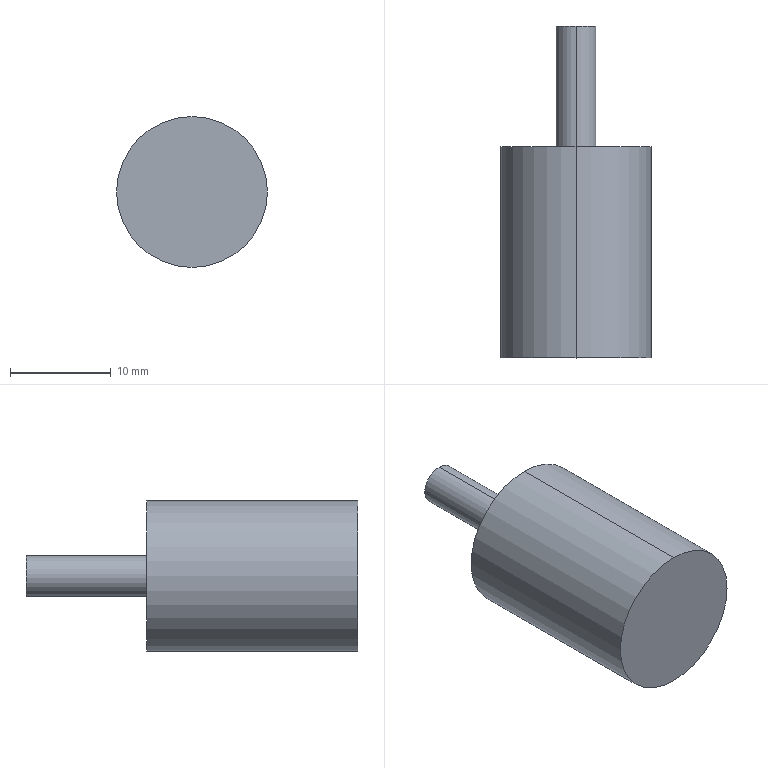Part | SolidWorks | features Revolution 1 | 1 solid | 7 faces | box 15 x 33 x 15 mm | volume 3862 mm3 | cylinder 4 | plane 3 | commonest cylinder face diameters 4 x2 15 x2
STEP:
#1=CARTESIAN_POINT('',(0.,-0.0007358,-0.0075));
#2=VERTEX_POINT('',#1);
#3=CARTESIAN_POINT('',(0.,-0.0007358,0.0075));
#4=VERTEX_POINT('',#3);
#5=CARTESIAN_POINT('',(0.,-0.0007358,0.));
#6=DIRECTION('',(0.,-1.,0.));
#7=DIRECTION('',(0.,0.,-1.));
#8=AXIS2_PLACEMENT_3D('',#5,#6,#7);
#9=CIRCLE('',#8,0.0075);
#10=EDGE_CURVE('',#2,#4,#9,.T.);
#11=ORIENTED_EDGE('',*,*,#10,.T.);
#12=CARTESIAN_POINT('',(0.,-0.02174,0.0075));
#13=VERTEX_POINT('',#12);
#14=CARTESIAN_POINT('',(0.,0.,0.0075));
#15=DIRECTION('',(0.,-1.,0.));
#16=VECTOR('',#15,1.);
#17=LINE('',#14,#16);
#18=EDGE_CURVE('',#4,#13,#17,.T.);
#19=ORIENTED_EDGE('',*,*,#18,.T.);
#20=CARTESIAN_POINT('',(0.,-0.02174,-0.0075));
#21=VERTEX_POINT('',#20);
#22=CARTESIAN_POINT('',(0.,-0.02174,0.));
#23=DIRECTION('',(0.,-1.,0.));
#24=DIRECTION('',(0.,0.,-1.));
#25=AXIS2_PLACEMENT_3D('',#22,#23,#24);
#26=CIRCLE('',#25,0.0075);
#27=EDGE_CURVE('',#21,#13,#26,.T.);
#28=ORIENTED_EDGE('',*,*,#27,.F.);
#29=CARTESIAN_POINT('',(0.,0.,-0.0075));
#30=DIRECTION('',(0.,-1.,0.));
#31=VECTOR('',#30,1.);
#32=LINE('',#29,#31);
#33=EDGE_CURVE('',#2,#21,#32,.T.);
#34=ORIENTED_EDGE('',*,*,#33,.F.);
#35=EDGE_LOOP('',(#11,#19,#28,#34));
#36=FACE_OUTER_BOUND('',#35,.T.);
#37=CARTESIAN_POINT('',(0.,0.,0.));
#38=DIRECTION('',(0.,-1.,0.));
#39=DIRECTION('',(0.,0.,-1.));
#40=AXIS2_PLACEMENT_3D('',#37,#38,#39);
#41=CYLINDRICAL_SURFACE('',#40,0.0075);
#42=ADVANCED_FACE('',(#36),#41,.T.);
#43=CARTESIAN_POINT('',(0.,0.01126,-0.002));
#44=VERTEX_POINT('',#43);
#45=CARTESIAN_POINT('',(0.,0.01126,0.002));
#46=VERTEX_POINT('',#45);
#47=CARTESIAN_POINT('',(0.,0.01126,0.));
#48=DIRECTION('',(0.,-1.,0.));
#49=DIRECTION('',(0.,0.,-1.));
#50=AXIS2_PLACEMENT_3D('',#47,#48,#49);
#51=CIRCLE('',#50,0.002);
#52=EDGE_CURVE('',#44,#46,#51,.T.);
#53=ORIENTED_EDGE('',*,*,#52,.T.);
#54=CARTESIAN_POINT('',(0.,-0.0007358,0.002));
#55=VERTEX_POINT('',#54);
#56=CARTESIAN_POINT('',(0.,0.,0.002));
#57=DIRECTION('',(0.,-1.,0.));
#58=VECTOR('',#57,1.);
#59=LINE('',#56,#58);
#60=EDGE_CURVE('',#46,#55,#59,.T.);
#61=ORIENTED_EDGE('',*,*,#60,.T.);
#62=CARTESIAN_POINT('',(0.,-0.0007358,-0.002));
#63=VERTEX_POINT('',#62);
#64=CARTESIAN_POINT('',(0.,-0.0007358,0.));
#65=DIRECTION('',(0.,-1.,0.));
#66=DIRECTION('',(0.,0.,-1.));
#67=AXIS2_PLACEMENT_3D('',#64,#65,#66);
#68=CIRCLE('',#67,0.002);
#69=EDGE_CURVE('',#63,#55,#68,.T.);
#70=ORIENTED_EDGE('',*,*,#69,.F.);
#71=CARTESIAN_POINT('',(0.,0.,-0.002));
#72=DIRECTION('',(0.,-1.,0.));
#73=VECTOR('',#72,1.);
#74=LINE('',#71,#73);
#75=EDGE_CURVE('',#44,#63,#74,.T.);
#76=ORIENTED_EDGE('',*,*,#75,.F.);
#77=EDGE_LOOP('',(#53,#61,#70,#76));
#78=FACE_OUTER_BOUND('',#77,.T.);
#79=CARTESIAN_POINT('',(0.,0.,0.));
#80=DIRECTION('',(0.,-1.,0.));
#81=DIRECTION('',(0.,0.,-1.));
#82=AXIS2_PLACEMENT_3D('',#79,#80,#81);
#83=CYLINDRICAL_SURFACE('',#82,0.002);
#84=ADVANCED_FACE('',(#78),#83,.T.);
#85=ORIENTED_EDGE('',*,*,#52,.F.);
#86=CARTESIAN_POINT('',(0.,0.01126,0.));
#87=DIRECTION('',(0.,-1.,0.));
#88=DIRECTION('',(0.,0.,-1.));
#89=AXIS2_PLACEMENT_3D('',#86,#87,#88);
#90=CIRCLE('',#89,0.002);
#91=EDGE_CURVE('',#46,#44,#90,.T.);
#92=ORIENTED_EDGE('',*,*,#91,.F.);
#93=EDGE_LOOP('',(#85,#92));
#94=FACE_OUTER_BOUND('',#93,.T.);
#95=CARTESIAN_POINT('',(0.,0.01126,0.));
#96=DIRECTION('',(0.,1.,0.));
#97=DIRECTION('',(0.,0.,1.));
#98=AXIS2_PLACEMENT_3D('',#95,#96,#97);
#99=PLANE('',#98);
#100=ADVANCED_FACE('',(#94),#99,.T.);
#101=ORIENTED_EDGE('',*,*,#60,.F.);
#102=ORIENTED_EDGE('',*,*,#91,.T.);
#103=ORIENTED_EDGE('',*,*,#75,.T.);
#104=CARTESIAN_POINT('',(0.,-0.0007358,0.));
#105=DIRECTION('',(0.,-1.,0.));
#106=DIRECTION('',(0.,0.,-1.));
#107=AXIS2_PLACEMENT_3D('',#104,#105,#106);
#108=CIRCLE('',#107,0.002);
#109=EDGE_CURVE('',#55,#63,#108,.T.);
#110=ORIENTED_EDGE('',*,*,#109,.F.);
#111=EDGE_LOOP('',(#101,#102,#103,#110));
#112=FACE_OUTER_BOUND('',#111,.T.);
#113=CARTESIAN_POINT('',(0.,0.,0.));
#114=DIRECTION('',(0.,-1.,0.));
#115=DIRECTION('',(0.,0.,-1.));
#116=AXIS2_PLACEMENT_3D('',#113,#114,#115);
#117=CYLINDRICAL_SURFACE('',#116,0.002);
#118=ADVANCED_FACE('',(#112),#117,.T.);
#119=ORIENTED_EDGE('',*,*,#69,.T.);
#120=ORIENTED_EDGE('',*,*,#109,.T.);
#121=EDGE_LOOP('',(#119,#120));
#122=FACE_BOUND('',#121,.T.);
#123=ORIENTED_EDGE('',*,*,#10,.F.);
#124=CARTESIAN_POINT('',(0.,-0.0007358,0.));
#125=DIRECTION('',(0.,-1.,0.));
#126=DIRECTION('',(0.,0.,-1.));
#127=AXIS2_PLACEMENT_3D('',#124,#125,#126);
#128=CIRCLE('',#127,0.0075);
#129=EDGE_CURVE('',#4,#2,#128,.T.);
#130=ORIENTED_EDGE('',*,*,#129,.F.);
#131=EDGE_LOOP('',(#123,#130));
#132=FACE_OUTER_BOUND('',#131,.T.);
#133=CARTESIAN_POINT('',(0.002,-0.0007358,0.));
#134=DIRECTION('',(0.,1.,0.));
#135=DIRECTION('',(0.,0.,1.));
#136=AXIS2_PLACEMENT_3D('',#133,#134,#135);
#137=PLANE('',#136);
#138=ADVANCED_FACE('',(#122,#132),#137,.T.);
#139=ORIENTED_EDGE('',*,*,#18,.F.);
#140=ORIENTED_EDGE('',*,*,#129,.T.);
#141=ORIENTED_EDGE('',*,*,#33,.T.);
#142=CARTESIAN_POINT('',(0.,-0.02174,0.));
#143=DIRECTION('',(0.,-1.,0.));
#144=DIRECTION('',(0.,0.,-1.));
#145=AXIS2_PLACEMENT_3D('',#142,#143,#144);
#146=CIRCLE('',#145,0.0075);
#147=EDGE_CURVE('',#13,#21,#146,.T.);
#148=ORIENTED_EDGE('',*,*,#147,.F.);
#149=EDGE_LOOP('',(#139,#140,#141,#148));
#150=FACE_OUTER_BOUND('',#149,.T.);
#151=CARTESIAN_POINT('',(0.,0.,0.));
#152=DIRECTION('',(0.,-1.,0.));
#153=DIRECTION('',(0.,0.,-1.));
#154=AXIS2_PLACEMENT_3D('',#151,#152,#153);
#155=CYLINDRICAL_SURFACE('',#154,0.0075);
#156=ADVANCED_FACE('',(#150),#155,.T.);
#157=ORIENTED_EDGE('',*,*,#27,.T.);
#158=ORIENTED_EDGE('',*,*,#147,.T.);
#159=EDGE_LOOP('',(#157,#158));
#160=FACE_OUTER_BOUND('',#159,.T.);
#161=CARTESIAN_POINT('',(0.0075,-0.02174,0.));
#162=DIRECTION('',(0.,-1.,0.));
#163=DIRECTION('',(0.,0.,-1.));
#164=AXIS2_PLACEMENT_3D('',#161,#162,#163);
#165=PLANE('',#164);
#166=ADVANCED_FACE('',(#160),#165,.T.);
#167=CLOSED_SHELL('',(#42,#84,#100,#118,#138,#156,#166));
#168=MANIFOLD_SOLID_BREP('',#167);
#169=CARTESIAN_POINT('',(0.,0.,0.));
#170=DIRECTION('',(0.,0.,1.));
#171=DIRECTION('',(1.,0.,0.));
#172=AXIS2_PLACEMENT_3D('',#169,#170,#171);
#173=(LENGTH_UNIT()NAMED_UNIT(*)SI_UNIT($,.METRE.));
#174=UNCERTAINTY_MEASURE_WITH_UNIT(LENGTH_MEASURE(0.00001),#173,'','');
#175=(NAMED_UNIT(*)PLANE_ANGLE_UNIT()SI_UNIT($,.RADIAN.));
#176=(NAMED_UNIT(*)SI_UNIT($,.STERADIAN.)SOLID_ANGLE_UNIT());
#177=(GEOMETRIC_REPRESENTATION_CONTEXT(3)GLOBAL_UNCERTAINTY_ASSIGNED_CONTEXT((#174))GLOBAL_UNIT_ASSIGNED_CONTEXT((#173,#175,#176))REPRESENTATION_CONTEXT('',''));
#178=ADVANCED_BREP_SHAPE_REPRESENTATION('',(#168,#172),#177);